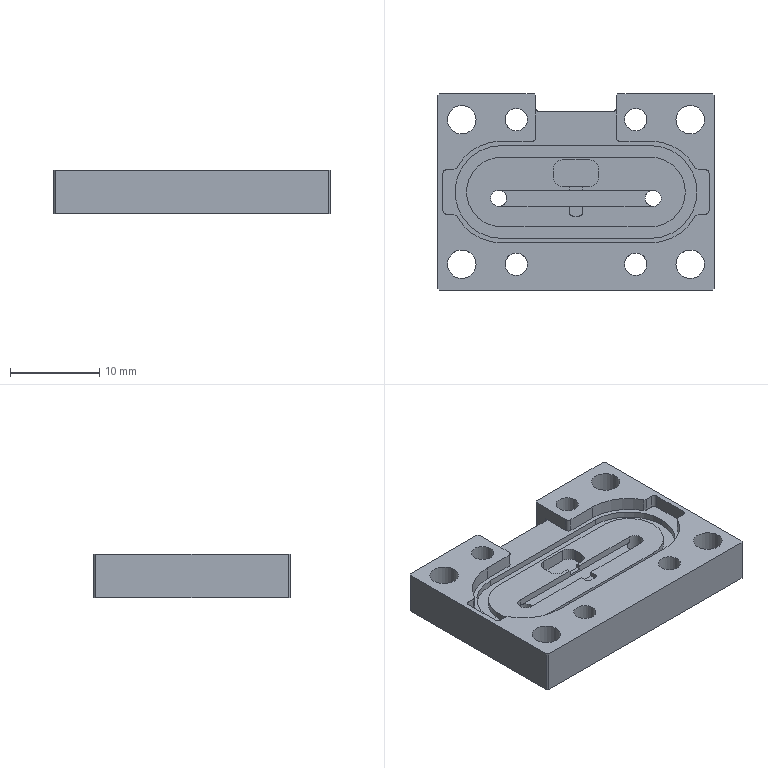NC program | NX | posted with a generic post | part box 31 x 22 x 4.9 mm
Lines 1 to 1660 of 7945, first 1453 of 1628 lines:
N10 G17 G21 G94 G90
(FACE_MILLING , TOOL : D50面刀)
N12 T12 M6
N14 G54
N16 G17 G0 G90 X43.5 Y0. S1600 M3
N18 G43 Z20. H12
N20 Z2.525
N22 G94 G1 Z0.525 F600.
N24 X40.5
N26 X-40.5
N28 X-43.5
N30 Z2.525
N32 G0 Z20.
N34 X43.5
N36 Z2.05
N38 G1 Z0.05
N40 X40.5
N42 X-40.5
N44 X-43.5
N46 Z2.05
N48 G0 Z20.
N50 M5
(ADAPTIVE_MILLING , TOOL : 6C-15L-25L)
N52 T02 M6
N54 G54
N56 G17 G0 G90 X-22.07 Y-0.418 S4500 M3
N58 G43 Z20. H2
N60 Z-2.9
N62 G94 G1 Z-5.9 F1500.
N64 X-21.095 Y-0.409
N66 G3 X-20.53 Y-0.006 R0.608
N68 X-20.23 Y2.844 R10.658
N70 G2 X-20.172 Y12.116 R798.279
N72 X-17.608 Y15.015 R3.885
N74 X-13.478 Y15.659 R12.183
N76 G1 X-7.365 Y15.7
N78 X16.28 Y15.698
N80 G2 X19.379 Y13.415 R3.673
N82 X20.139 Y9.502 R10.224
N84 X20.172 Y-12.09 R928.263
N86 X17.539 Y-15.024 R3.915
N88 X13.407 Y-15.647 R12.574
N90 G1 X7.369 Y-15.688
N92 X-16.328 Y-15.696
N94 G2 X-19.386 Y-13.414 R3.675
N96 X-20.146 Y-9.35 R10.554
N98 X-20.141 Y-0.409 R126.129
N100 G3 X-19.9 Y7.956 R92.469
N102 G2 X-19.829 Y11.214 R25.556
N104 X-16.647 Y14.675 R4.74
N106 X-11.881 Y15.361 R14.905
N108 G1 X-5.656 Y15.399
N110 X15.004 Y15.398
N112 G2 X19.076 Y12.392 R4.554
N114 X19.847 Y7.794 R13.145
N116 X19.876 Y-10.853 R799.951
N118 X16.799 Y-14.599 R4.632
N120 X12.304 Y-15.333 R13.408
N122 X5.592 Y-15.388 R559.777
N124 G1 X-15.015 Y-15.397
N126 G2 X-19.054 Y-12.451 R4.529
N128 X-19.846 Y-7.818 R12.948
N130 X-19.675 Y2.314 R100.736
N132 G1 X-19.576 Y9.907
N134 G2 X-16.059 Y14.284 R5.172
N136 X-11.378 Y15.039 R14.663
N138 X-3.804 Y15.099 R572.181
N140 G1 X13.955 Y15.097
N142 G2 X18.731 Y11.687 R5.128
N144 X19.534 Y6.98 R14.045
N146 X19.565 Y-9.99 R503.525
N148 X16.034 Y-14.277 R5.19
N150 X11.051 Y-15.036 R15.491
N152 G1 X3.777 Y-15.089
N154 X-13.961 Y-15.095
N156 G2 X-18.749 Y-11.651 R5.129
N158 X-19.543 Y-6.75 R14.635
N160 X-19.376 Y2.491 R107.625
N162 X-19.256 Y9.274 R367.832
N164 X-18.556 Y11.514 R6.868
N166 X-15.459 Y14.198 R3.677
N168 X-8.897 Y14.778 R31.595
N170 G1 X-2.597 Y14.799
N172 G2 X13.64 Y14.771 R937.515
N174 X16.022 Y14.055 R7.126
N176 X18.648 Y11.178 R3.618
N178 X19.278 Y4.359 R31.12
N180 X19.266 Y-9.177 R445.151
N182 X18.559 Y-11.492 R6.838
N184 X15.604 Y-14.161 R3.602
N186 X8.519 Y-14.77 R33.556
N188 G1 X3.419 Y-14.789
N190 X-12.915 Y-14.795
N192 G2 X-16.018 Y-14.056 R6.813
N194 X-18.698 Y-10.959 R3.68
N196 X-19.28 Y-4.022 R32.852
N198 X-19.034 Y4.585 R641.476
N200 X-18.917 Y8.867 R47.436
N202 G1 X-18.65 Y10.111
N204 G2 X-18.228 Y12.375 R3.99
N206 X-16.115 Y14.043 R3.859
N208 X-6.563 Y14.49 R80.605
N210 G1 X-1.538 Y14.499
N212 G2 X13.385 Y14.472 R874.725
N214 G1 X14.709 Y14.15
N216 G2 X16.045 Y14.052 R7.674
N218 G3 X16.699 Y14.816 R0.6
N220 X16.308 Y15.245 Z-5.85 R0.784
N222 G1 X15.815 Y15.573 Z-5.8
N224 X15.129 Y16.022
N226 X15.004 Y16.06
N228 X14.874 Y16.08
N230 X-14.033 Y16.171
N232 X-14.165 Y16.13
N234 X-14.289 Y16.068
N236 X-14.879 Y15.649
N238 X-15.23 Y15.408 Z-5.836
N240 X-15.563 Y15.142 Z-5.872
N242 X-15.653 Y15.001 Z-5.886
N244 X-15.704 Y14.842 Z-5.9
N246 G3 X-15.111 Y14.15 R0.6
N248 G1 X-3.186 Y14.197
N250 X12.714 Y14.198
N252 G3 X14.735 Y14.15 R11.377
N254 X14.943 Y15.313 R0.6
N256 G1 X13.797 Y15.63 Z-5.8
N258 X13.442 Y15.734
N260 X13.079 Y15.806
N262 X-7.985 Y15.8
N264 X-8.577 Y15.643
N266 X-9.723 Y15.327 Z-5.9
N268 G3 X-9.561 Y14.15 R0.6
N270 G1 X-4.698
N272 G3 X0.873 Y13.901 R37.444
N274 X3.621 Y13.934 R28.005
N276 G2 X4.702 Y14.15 R3.288
N278 G1 X13.064
N280 G3 X13.724 Y14.81 R0.66
N282 X13.058 Y15.47 R0.66
N284 G1 X4.434 Y15.389
N286 X3.245 Y15.377 Z-5.8
N288 X-3.054 Y15.318
N290 X-3.421 Z-5.831
N292 X-3.788 Y15.292 Z-5.862
N294 G3 X-4.16 Y15.049 Z-5.9 R0.678
N296 X-3.885 Y14.043 R0.66
N298 X-0.878 Y13.646 R9.579
N300 X2.956 Y13.646 R38.958
N302 G1 X3.093 Y13.706
N304 G3 X3.325 Y14.534 R0.661
N306 X2.657 Y14.92 Z-5.831 R0.697
N308 G1 X2.287 Y14.94 Z-5.8
N310 X-2.826 Y15.22
N312 X-3.211 Y15.244 Z-5.832
N314 X-3.596 Y15.245 Z-5.865
N316 G3 X-3.962 Y15.06 Z-5.9 R0.687
N318 X-3.746 Y13.985 R0.66
N320 X-0.769 Y13.391 R7.752
N322 X2.624 Y13.404 R16.695
N324 X3.125 Y13.728 R3.317
N326 G1 X3.645 Y13.943
N328 G3 X3.915 Y14.956 R0.66
N330 X3.262 Y15.21 Z-5.838 R0.713
N332 G1 X2.806 Y15.199 Z-5.8
N334 X-2.47 Y15.068
N336 X-2.826 Y15.063 Z-5.83
N338 X-3.181 Y15.029 Z-5.86
N340 G3 X-3.559 Y14.758 Z-5.9 R0.674
N342 X-3.261 Y13.784 R0.66
N344 X-0.251 Y13.116 R7.191
N346 X2.371 Y13.18 R8.911
N348 G1 X2.826 Y13.499
N350 G3 X3.017 Y14.314 R0.661
N352 X2.347 Y14.686 Z-5.832 R0.698
N354 G1 X1.971 Y14.703 Z-5.8
N356 X-2.179 Y14.888
N358 X-2.508 Y14.905 Z-5.828
N360 X-2.837 Y14.9 Z-5.856
N362 G3 X-3.27 Y14.62 Z-5.9 R0.669
N364 X-3.125 Y13.728 R0.661
N366 X-0.846 Y12.948 R4.437
N368 X2.118 Y12.95 R7.962
N370 X2.501 Y13.249 R3.333
N372 X2.698 Y14.052 R0.661
N374 X2.037 Y14.439 Z-5.832 R0.699
N376 G1 X1.66 Y14.465 Z-5.8
N378 X-1.954 Y14.714
N380 X-2.283 Y14.74 Z-5.828
N382 X-2.613 Y14.743 Z-5.856
N384 G3 X-3.052 Y14.475 Z-5.9 R0.669
N386 X-2.917 Y13.568 R0.661
N388 X-0.467 Y12.683 R4.638
N390 X2.018 Y12.784 R5.044
N392 G1 X2.334 Y13.085
N394 G3 X2.452 Y13.837 R0.662
N396 X1.802 Y14.212 Z-5.833 R0.704
N398 G1 X1.407 Y14.245 Z-5.8
N400 X-1.68 Y14.501
N402 X-2.007 Y14.531 Z-5.828
N404 X-2.337 Y14.538 Z-5.856
N406 G3 X-2.78 Y14.276 Z-5.9 R0.668
N408 X-2.649 Y13.363 R0.661
N410 X0.082 Y12.41 R4.757
N412 X1.904 Y12.62 R3.297
N414 G1 X2.175 Y12.911
N416 G3 X2.275 Y13.642 R0.662
N418 X1.629 Y14.019 Z-5.834 R0.705
N420 G1 X1.231 Y14.055 Z-5.8
N422 X-1.435 Y14.298
N424 X-1.759 Y14.33 Z-5.827
N426 X-2.085 Y14.339 Z-5.855
N428 G3 X-2.533 Y14.074 Z-5.9 R0.668
N430 X-2.472 Y13.226 R0.661
N432 X-0.241 Y12.252 R3.679
N434 X1.777 Y12.447 R3.122
N436 G1 X1.906 Y12.582
N438 G3 X1.934 Y13.214 R0.665
N440 X1.35 Y13.593 Z-5.839 R0.715
N442 G1 X0.896 Y13.679 Z-5.8
N444 X-1.217 Y14.079
N446 X-1.538 Y14.142 Z-5.828
N448 X-1.864 Y14.183 Z-5.855
N450 G3 X-2.333 Y13.966 Z-5.9 R0.668
N452 X-2.315 Y13.065 R0.661
N454 X-0.59 Y12.15 R2.983
N456 X1.471 Y12.211 R10.87
N458 X1.998 Y12.704 R1.047
N460 X2.074 Y13.424 R0.663
N462 X1.418 Y13.788 Z-5.833 R0.704
N464 G1 X1.022 Y13.814 Z-5.8
N466 X-1.099 Y13.955
N468 X-1.431 Y13.979 Z-5.828
N470 X-1.763 Y13.982 Z-5.856
N472 G3 X-2.199 Y13.718 Z-5.9 R0.669
N474 X-2.156 Y12.891 R0.661
N476 X-0.568 Y12.15 R1.703
N478 X-0.353 Y13.434 R0.66
N480 G1 X-1.382 Y13.78
N482 G3 X-2.004 Y12.712 R0.66
N484 X-1. Y12.15 R1.075
N486 X-0.759 Y13.425 R0.66
N488 G1 X-1.221 Y13.595
N490 G3 X-1.927 Y12.617 R0.66
N492 X-1.224 Y12.15 R0.744
N494 X-1.896 Y13.122 R-0.713
N496 X-1.851 Y12.487 R0.727
N498 X-1.299 Y12.15 R0.666
N500 G1 X1.427 Y12.163
N502 G3 X1.852 Y12.489 R0.739
N504 X1.912 Y12.953 R0.615
N506 G1 X1.839 Y13.214
N508 X1.521 Y14.359 Z-5.8
N510 G2 X1.852 Y15.165 R0.613
N512 G1 X2.711 Y15.512
N514 X3.584 Y15.822
N516 X3.944 Y15.906
N518 X4.31 Y15.951
N520 X7.639 Y16.145
N522 X10.969 Y16.318
N524 G2 X15.315 Y16.024 R22.708
N526 G1 X16.999 Y15.737
N528 G2 X18.51 Y14.907 R3.241
N530 G1 X19.297 Y14.13
N532 G2 X19.318 Y13.431 R0.619
N534 G1 X18.796 Y12.362 Z-5.9
N536 X18.655 Y12.083
N538 G3 X18.543 Y11.615 R1.223
N540 G2 X18.99 Y1.939 R81.107
N542 X18.972 Y-8.859 R673.915
N544 G1 X18.65 Y-10.196
N546 G2 X18.557 Y-11.508 R7.62
N548 G3 X19.321 Y-12.162 R0.6
N550 X19.75 Y-11.771 Z-5.85 R0.784
N552 G1 X20.078 Y-11.277 Z-5.8
N554 X20.527 Y-10.591
N556 X20.565 Y-10.466
N558 X20.585 Y-10.337
N560 X20.671 Y9.495
N562 X20.63 Y9.628
N564 X20.567 Y9.752
N566 X20.149 Y10.342
N568 X19.908 Y10.693 Z-5.836
N570 X19.642 Y11.025 Z-5.872
N572 X19.501 Y11.115 Z-5.886
N574 X19.342 Y11.166 Z-5.9
N576 G3 X18.65 Y10.573 R0.6
N578 G1 X18.697 Y-1.545
N580 G2 X18.65 Y-10.203 R441.565
N582 G3 X19.813 Y-10.412 R0.6
N584 G1 X20.13 Y-9.266 Z-5.8
N586 X20.234 Y-8.911
N588 X20.306 Y-8.548
N590 X20.3 Y3.373
N592 X20.143 Y3.964
N594 X19.828 Y5.111 Z-5.9
N596 G3 X18.65 Y4.948 R0.6
N598 G1 Y-10.802
N600 G2 X14.91 Y-14.153 R3.498
N602 X3.692 Y-14.481 R128.863
N604 G1 X-0.808 Y-14.491
N606 G2 X-13.363 Y-14.47 R602.67
N608 G1 X-14.703 Y-14.15
N610 G2 X-16.045 Y-14.052 R7.665
N612 G3 X-16.699 Y-14.816 R0.6
N614 X-16.308 Y-15.245 Z-5.85 R0.784
N616 G1 X-15.815 Y-15.573 Z-5.8
N618 X-15.129 Y-16.022
N620 X-15.004 Y-16.06
N622 X-14.874 Y-16.08
N624 X13.92 Y-16.171
N626 X14.053 Y-16.13
N628 X14.176 Y-16.068
N630 X14.767 Y-15.649
N632 X15.118 Y-15.408 Z-5.836
N634 X15.45 Y-15.142 Z-5.872
N636 X15.54 Y-15.001 Z-5.886
N638 X15.591 Y-14.842 Z-5.9
N640 G3 X14.998 Y-14.15 R0.6
N642 G1 X-0.945 Y-14.19
N644 G2 X-14.706 Y-14.15 R831.508
N646 G3 X-14.915 Y-15.313 R0.6
N648 G1 X-13.769 Y-15.63 Z-5.8
N650 X-13.413 Y-15.734
N652 X-13.051 Y-15.806
N654 X4.273 Y-15.8
N656 X4.864 Y-15.643
N658 X6.011 Y-15.328 Z-5.9
N660 G3 X5.848 Y-14.15 R0.6
N662 G1 X-15.302
N664 G2 X-18.657 Y-10.406 R3.505
N666 X-18.81 Y1.708 R84.207
N668 G3 X-18.65 Y10.14 R365.879
N670 X-19.815 Y10.341 R0.6
N672 G1 X-20.13 Y9.194 Z-5.8
N674 X-20.231 Y8.842
N676 X-20.306 Y8.484
N678 X-20.678 Y-9.442
N680 X-20.65 Y-9.631
N682 X-20.566 Y-9.803
N684 X-20.152 Y-10.383
N686 X-19.908 Y-10.733 Z-5.836
N688 X-19.64 Y-11.066 Z-5.872
N690 X-19.5 Y-11.155 Z-5.886
N692 X-19.342 Y-11.205 Z-5.9
N694 G3 X-18.65 Y-10.613 R0.6
N696 G1 Y7.988
N698 G3 X-19.36 Y8.584 R0.606
N700 G1 X-20.137 Y8.449
N702 Z-2.9
N704 G0 Z20.
N706 M5
(DRILLING , TOOL : D5点钻)
N708 T07 M6
N710 G54
N712 G17 G0 G90 X-12.8 Y8.1 S1200 M3
N714 G43 Z20. H7
N716 G94 G81 G99 Z-1. F100. R3.
N718 X-6.7
N720 X6.7
N722 X12.8
N724 Y-8.1
N726 X6.7
N728 X-6.7
N730 X-12.8
N732 G80
N734 G0 X-12.8 Y-8.1 Z20.
N736 M5
(DRILLING_1 , TOOL : D3.2钻头)
N738 T08 M6
N740 G54
N742 G17 G0 G90 X-12.8 Y8.1 S1600 M3
N744 G43 Z20. H8
N746 G94 G83 G99 Z-7.361 F80. Q1. R3.
N748 Y-8.1
N750 X12.8
N752 Y8.1
N754 G80
N756 G0 X12.8 Y8.1 Z20.
N758 M5
(DRILLING_2 , TOOL : D2.5钻头)
N760 T13 M6
N762 G54
N764 G17 G0 G90 X-6.7 Y8.1 S3000 M3
N766 G43 Z20. H13
N768 G94 G81 G99 Z-6.5 F60. R3.
N770 X6.7
N772 Y-8.1
N774 X-6.7
N776 G80
N778 G0 X-6.7 Y-8.1 Z20.
N780 M5
(DRILLING_COPY , TOOL : D5点钻)
N782 T07 M6
N784 G54
N786 G17 G0 G90 X-12.8 Y8.1 S2000 M3
N788 G43 Z20. H7
N790 G94 G81 G99 Z-1.6 F80. R3.
N792 X12.8
N794 Y-8.1
N796 X-12.8
N798 G80
N800 G0 X-12.8 Y-8.1 Z20.
(DRILLING_COPY_1 , TOOL : D5点钻)
N802 X-6.7 Y8.1
N804 G81 Z-1.4 F80. R3.
N806 X6.7
N808 Y-8.1
N810 X-6.7
N812 G80
N814 G0 X-6.7 Y-8.1 Z20.
N816 M5
(THREAD_MILLING , TOOL : 螺纹铣刀M3)
N818 T14 M6
N820 G54
N822 G17 G0 G90 X-6.7 Y8.1 S3500 M3
N824 G43 Z20. H14
N826 Z0.625
N828 G42 G94 G1 X-6.713 Y8.035 Z0.583 F80. D14
N830 X-6.788 Z0.542
N832 X-6.8 Y8.1 Z0.5
N834 G2 X-6.8 Y8.1 Z0. I0.1 J0.
N836 X-6.8 Y8.1 Z-0.5 I0.1 J0.
N838 X-6.8 Y8.1 Z-1. I0.1 J0.
N840 X-6.8 Y8.1 Z-1.5 I0.1 J0.
N842 X-6.8 Y8.1 Z-2. I0.1 J0.
N844 X-6.8 Y8.1 Z-2.5 I0.1 J0.
N846 X-6.8 Y8.1 Z-3. I0.1 J0.
N848 X-6.8 Y8.1 Z-3.5 I0.1 J0.
N850 X-6.8 Y8.1 Z-4. I0.1 J0.
N852 X-6.8 Y8.1 Z-4.5 I0.1 J0.
N854 X-6.8 Y8.1 Z-5. I0.1 J0.
N856 X-6.8 Y8.1 Z-5.5 I0.1 J0.
N858 X-6.731 Y8.195 Z-5.6 R0.1
N860 G1 X-6.665 Y8.203 Z-5.642
N862 X-6.642 Y8.132 Z-5.683
N864 X-6.7 Y8.1 Z-5.725
N866 G40
N868 G0 Z20.
N870 Z0.547
N872 G42 G1 X-6.789 Y8.055
N874 X-6.826 Y8.033 Z0.531
N876 X-6.86 Y8.059 Z0.516
N878 X-6.85 Y8.1 Z0.5
N880 G2 X-6.85 Y8.1 Z0. I0.15 J0.
N882 X-6.85 Y8.1 Z-0.5 I0.15 J0.
N884 X-6.85 Y8.1 Z-1. I0.15 J0.
N886 X-6.85 Y8.1 Z-1.5 I0.15 J0.
N888 X-6.85 Y8.1 Z-2. I0.15 J0.
N890 X-6.85 Y8.1 Z-2.5 I0.15 J0.
N892 X-6.85 Y8.1 Z-3. I0.15 J0.
N894 X-6.85 Y8.1 Z-3.5 I0.15 J0.
N896 X-6.85 Y8.1 Z-4. I0.15 J0.
N898 X-6.85 Y8.1 Z-4.5 I0.15 J0.
N900 X-6.85 Y8.1 Z-5. I0.15 J0.
N902 X-6.85 Y8.1 Z-5.5 I0.15 J0.
N904 X-6.746 Y8.243 Z-5.6 R0.15
N906 G1 X-6.71 Y8.265 Z-5.616
N908 X-6.675 Y8.24 Z-5.631
N910 X-6.685 Y8.199 Z-5.647
N912 G40
N914 X-6.7 Y8.1
N916 G0 Z20.
N918 Z0.57
N920 G42 G1 X-6.773 Y8.031
N922 X-6.833 Y7.989 Z0.547
N924 X-6.902 Y8.026 Z0.523
N926 X-6.9 Y8.1 Z0.5
N928 G2 X-6.9 Y8.1 Z0. I0.2 J0.
N930 X-6.9 Y8.1 Z-0.5 I0.2 J0.
N932 X-6.9 Y8.1 Z-1. I0.2 J0.
N934 X-6.9 Y8.1 Z-1.5 I0.2 J0.
N936 X-6.9 Y8.1 Z-2. I0.2 J0.
N938 X-6.9 Y8.1 Z-2.5 I0.2 J0.
N940 X-6.9 Y8.1 Z-3. I0.2 J0.
N942 X-6.9 Y8.1 Z-3.5 I0.2 J0.
N944 X-6.9 Y8.1 Z-4. I0.2 J0.
N946 X-6.9 Y8.1 Z-4.5 I0.2 J0.
N948 X-6.9 Y8.1 Z-5. I0.2 J0.
N950 X-6.9 Y8.1 Z-5.5 I0.2 J0.
N952 X-6.762 Y8.29 Z-5.6 R0.2
N954 G1 X-6.692 Y8.315 Z-5.623
N956 X-6.635 Y8.261 Z-5.647
N958 X-6.657 Y8.19 Z-5.67
N960 G40
N962 X-6.7 Y8.1
N964 G0 Z20.
N966 Z0.584
N968 G42 G1 X-6.759 Y8.019
N970 G2 X-6.95 Y8.1 Z0.5 R0.113
N972 X-6.95 Y8.1 Z0. I0.25 J0.
N974 X-6.95 Y8.1 Z-0.5 I0.25 J0.
N976 X-6.95 Y8.1 Z-1. I0.25 J0.
N978 X-6.95 Y8.1 Z-1.5 I0.25 J0.
N980 X-6.95 Y8.1 Z-2. I0.25 J0.
N982 X-6.95 Y8.1 Z-2.5 I0.25 J0.
N984 X-6.95 Y8.1 Z-3. I0.25 J0.
N986 X-6.95 Y8.1 Z-3.5 I0.25 J0.
N988 X-6.95 Y8.1 Z-4. I0.25 J0.
N990 X-6.95 Y8.1 Z-4.5 I0.25 J0.
N992 X-6.95 Y8.1 Z-5. I0.25 J0.
N994 X-6.95 Y8.1 Z-5.5 I0.25 J0.
N996 X-6.777 Y8.338 Z-5.6 R0.25
N998 X-6.641 Y8.181 Z-5.684 R0.113
N1000 G40
N1002 G1 X-6.7 Y8.1
N1004 G0 Z20.
N1006 X6.7
N1008 Z0.625
N1010 G42 G1 X6.713 Y8.165 Z0.583
N1012 X6.788 Z0.542
N1014 X6.8 Y8.1 Z0.5
N1016 G2 X6.8 Y8.1 Z0. I-0.1 J0.
N1018 X6.8 Y8.1 Z-0.5 I-0.1 J0.
N1020 X6.8 Y8.1 Z-1. I-0.1 J0.
N1022 X6.8 Y8.1 Z-1.5 I-0.1 J0.
N1024 X6.8 Y8.1 Z-2. I-0.1 J0.
N1026 X6.8 Y8.1 Z-2.5 I-0.1 J0.
N1028 X6.8 Y8.1 Z-3. I-0.1 J0.
N1030 X6.8 Y8.1 Z-3.5 I-0.1 J0.
N1032 X6.8 Y8.1 Z-4. I-0.1 J0.
N1034 X6.8 Y8.1 Z-4.5 I-0.1 J0.
N1036 X6.8 Y8.1 Z-5. I-0.1 J0.
N1038 X6.8 Y8.1 Z-5.5 I-0.1 J0.
N1040 X6.731 Y8.005 Z-5.6 R0.1
N1042 G1 X6.665 Y7.997 Z-5.642
N1044 X6.642 Y8.068 Z-5.683
N1046 X6.7 Y8.1 Z-5.725
N1048 G40
N1050 G0 Z20.
N1052 Z0.547
N1054 G42 G1 X6.789 Y8.145
N1056 X6.826 Y8.167 Z0.531
N1058 X6.86 Y8.141 Z0.516
N1060 X6.85 Y8.1 Z0.5
N1062 G2 X6.85 Y8.1 Z0. I-0.15 J0.
N1064 X6.85 Y8.1 Z-0.5 I-0.15 J0.
N1066 X6.85 Y8.1 Z-1. I-0.15 J0.
N1068 X6.85 Y8.1 Z-1.5 I-0.15 J0.
N1070 X6.85 Y8.1 Z-2. I-0.15 J0.
N1072 X6.85 Y8.1 Z-2.5 I-0.15 J0.
N1074 X6.85 Y8.1 Z-3. I-0.15 J0.
N1076 X6.85 Y8.1 Z-3.5 I-0.15 J0.
N1078 X6.85 Y8.1 Z-4. I-0.15 J0.
N1080 X6.85 Y8.1 Z-4.5 I-0.15 J0.
N1082 X6.85 Y8.1 Z-5. I-0.15 J0.
N1084 X6.85 Y8.1 Z-5.5 I-0.15 J0.
N1086 X6.746 Y7.957 Z-5.6 R0.15
N1088 G1 X6.71 Y7.935 Z-5.616
N1090 X6.675 Y7.96 Z-5.631
N1092 X6.685 Y8.001 Z-5.647
N1094 G40
N1096 X6.7 Y8.1
N1098 G0 Z20.
N1100 Z0.57
N1102 G42 G1 X6.773 Y8.169
N1104 X6.833 Y8.211 Z0.547
N1106 X6.902 Y8.174 Z0.523
N1108 X6.9 Y8.1 Z0.5
N1110 G2 X6.9 Y8.1 Z0. I-0.2 J0.
N1112 X6.9 Y8.1 Z-0.5 I-0.2 J0.
N1114 X6.9 Y8.1 Z-1. I-0.2 J0.
N1116 X6.9 Y8.1 Z-1.5 I-0.2 J0.
N1118 X6.9 Y8.1 Z-2. I-0.2 J0.
N1120 X6.9 Y8.1 Z-2.5 I-0.2 J0.
N1122 X6.9 Y8.1 Z-3. I-0.2 J0.
N1124 X6.9 Y8.1 Z-3.5 I-0.2 J0.
N1126 X6.9 Y8.1 Z-4. I-0.2 J0.
N1128 X6.9 Y8.1 Z-4.5 I-0.2 J0.
N1130 X6.9 Y8.1 Z-5. I-0.2 J0.
N1132 X6.9 Y8.1 Z-5.5 I-0.2 J0.
N1134 X6.762 Y7.91 Z-5.6 R0.2
N1136 G1 X6.692 Y7.885 Z-5.623
N1138 X6.635 Y7.939 Z-5.647
N1140 X6.657 Y8.01 Z-5.67
N1142 G40
N1144 X6.7 Y8.1
N1146 G0 Z20.
N1148 Z0.584
N1150 G42 G1 X6.759 Y8.181
N1152 G2 X6.95 Y8.1 Z0.5 R0.113
N1154 X6.95 Y8.1 Z0. I-0.25 J0.
N1156 X6.95 Y8.1 Z-0.5 I-0.25 J0.
N1158 X6.95 Y8.1 Z-1. I-0.25 J0.
N1160 X6.95 Y8.1 Z-1.5 I-0.25 J0.
N1162 X6.95 Y8.1 Z-2. I-0.25 J0.
N1164 X6.95 Y8.1 Z-2.5 I-0.25 J0.
N1166 X6.95 Y8.1 Z-3. I-0.25 J0.
N1168 X6.95 Y8.1 Z-3.5 I-0.25 J0.
N1170 X6.95 Y8.1 Z-4. I-0.25 J0.
N1172 X6.95 Y8.1 Z-4.5 I-0.25 J0.
N1174 X6.95 Y8.1 Z-5. I-0.25 J0.
N1176 X6.95 Y8.1 Z-5.5 I-0.25 J0.
N1178 X6.777 Y7.862 Z-5.6 R0.25
N1180 X6.641 Y8.019 Z-5.684 R0.113
N1182 G40
N1184 G1 X6.7 Y8.1
N1186 G0 Z20.
N1188 Y-8.1
N1190 Z0.625
N1192 G42 G1 X6.713 Y-8.035 Z0.583
N1194 X6.788 Z0.542
N1196 X6.8 Y-8.1 Z0.5
N1198 G2 X6.8 Y-8.1 Z0. I-0.1 J0.
N1200 X6.8 Y-8.1 Z-0.5 I-0.1 J0.
N1202 X6.8 Y-8.1 Z-1. I-0.1 J0.
N1204 X6.8 Y-8.1 Z-1.5 I-0.1 J0.
N1206 X6.8 Y-8.1 Z-2. I-0.1 J0.
N1208 X6.8 Y-8.1 Z-2.5 I-0.1 J0.
N1210 X6.8 Y-8.1 Z-3. I-0.1 J0.
N1212 X6.8 Y-8.1 Z-3.5 I-0.1 J0.
N1214 X6.8 Y-8.1 Z-4. I-0.1 J0.
N1216 X6.8 Y-8.1 Z-4.5 I-0.1 J0.
N1218 X6.8 Y-8.1 Z-5. I-0.1 J0.
N1220 X6.8 Y-8.1 Z-5.5 I-0.1 J0.
N1222 X6.731 Y-8.195 Z-5.6 R0.1
N1224 G1 X6.665 Y-8.203 Z-5.642
N1226 X6.642 Y-8.132 Z-5.683
N1228 X6.7 Y-8.1 Z-5.725
N1230 G40
N1232 G0 Z20.
N1234 Z0.547
N1236 G42 G1 X6.789 Y-8.055
N1238 X6.826 Y-8.033 Z0.531
N1240 X6.86 Y-8.059 Z0.516
N1242 X6.85 Y-8.1 Z0.5
N1244 G2 X6.85 Y-8.1 Z0. I-0.15 J0.
N1246 X6.85 Y-8.1 Z-0.5 I-0.15 J0.
N1248 X6.85 Y-8.1 Z-1. I-0.15 J0.
N1250 X6.85 Y-8.1 Z-1.5 I-0.15 J0.
N1252 X6.85 Y-8.1 Z-2. I-0.15 J0.
N1254 X6.85 Y-8.1 Z-2.5 I-0.15 J0.
N1256 X6.85 Y-8.1 Z-3. I-0.15 J0.
N1258 X6.85 Y-8.1 Z-3.5 I-0.15 J0.
N1260 X6.85 Y-8.1 Z-4. I-0.15 J0.
N1262 X6.85 Y-8.1 Z-4.5 I-0.15 J0.
N1264 X6.85 Y-8.1 Z-5. I-0.15 J0.
N1266 X6.85 Y-8.1 Z-5.5 I-0.15 J0.
N1268 X6.746 Y-8.243 Z-5.6 R0.15
N1270 G1 X6.71 Y-8.265 Z-5.616
N1272 X6.675 Y-8.24 Z-5.631
N1274 X6.685 Y-8.199 Z-5.647
N1276 G40
N1278 X6.7 Y-8.1
N1280 G0 Z20.
N1282 Z0.57
N1284 G42 G1 X6.773 Y-8.031
N1286 X6.833 Y-7.989 Z0.547
N1288 X6.902 Y-8.026 Z0.523
N1290 X6.9 Y-8.1 Z0.5
N1292 G2 X6.9 Y-8.1 Z0. I-0.2 J0.
N1294 X6.9 Y-8.1 Z-0.5 I-0.2 J0.
N1296 X6.9 Y-8.1 Z-1. I-0.2 J0.
N1298 X6.9 Y-8.1 Z-1.5 I-0.2 J0.
N1300 X6.9 Y-8.1 Z-2. I-0.2 J0.
N1302 X6.9 Y-8.1 Z-2.5 I-0.2 J0.
N1304 X6.9 Y-8.1 Z-3. I-0.2 J0.
N1306 X6.9 Y-8.1 Z-3.5 I-0.2 J0.
N1308 X6.9 Y-8.1 Z-4. I-0.2 J0.
N1310 X6.9 Y-8.1 Z-4.5 I-0.2 J0.
N1312 X6.9 Y-8.1 Z-5. I-0.2 J0.
N1314 X6.9 Y-8.1 Z-5.5 I-0.2 J0.
N1316 X6.762 Y-8.29 Z-5.6 R0.2
N1318 G1 X6.692 Y-8.315 Z-5.623
N1320 X6.635 Y-8.261 Z-5.647
N1322 X6.657 Y-8.19 Z-5.67
N1324 G40
N1326 X6.7 Y-8.1
N1328 G0 Z20.
N1330 Z0.584
N1332 G42 G1 X6.759 Y-8.019
N1334 G2 X6.95 Y-8.1 Z0.5 R0.113
N1336 X6.95 Y-8.1 Z0. I-0.25 J0.
N1338 X6.95 Y-8.1 Z-0.5 I-0.25 J0.
N1340 X6.95 Y-8.1 Z-1. I-0.25 J0.
N1342 X6.95 Y-8.1 Z-1.5 I-0.25 J0.
N1344 X6.95 Y-8.1 Z-2. I-0.25 J0.
N1346 X6.95 Y-8.1 Z-2.5 I-0.25 J0.
N1348 X6.95 Y-8.1 Z-3. I-0.25 J0.
N1350 X6.95 Y-8.1 Z-3.5 I-0.25 J0.
N1352 X6.95 Y-8.1 Z-4. I-0.25 J0.
N1354 X6.95 Y-8.1 Z-4.5 I-0.25 J0.
N1356 X6.95 Y-8.1 Z-5. I-0.25 J0.
N1358 X6.95 Y-8.1 Z-5.5 I-0.25 J0.
N1360 X6.777 Y-8.338 Z-5.6 R0.25
N1362 X6.641 Y-8.181 Z-5.684 R0.113
N1364 G40
N1366 G1 X6.7 Y-8.1
N1368 G0 Z20.
N1370 X-6.7
N1372 Z0.625
N1374 G42 G1 X-6.688 Y-8.035 Z0.583
N1376 X-6.613 Z0.542
N1378 X-6.6 Y-8.1 Z0.5
N1380 G2 X-6.6 Y-8.1 Z0. I-0.1 J0.
N1382 X-6.6 Y-8.1 Z-0.5 I-0.1 J0.
N1384 X-6.6 Y-8.1 Z-1. I-0.1 J0.
N1386 X-6.6 Y-8.1 Z-1.5 I-0.1 J0.
N1388 X-6.6 Y-8.1 Z-2. I-0.1 J0.
N1390 X-6.6 Y-8.1 Z-2.5 I-0.1 J0.
N1392 X-6.6 Y-8.1 Z-3. I-0.1 J0.
N1394 X-6.6 Y-8.1 Z-3.5 I-0.1 J0.
N1396 X-6.6 Y-8.1 Z-4. I-0.1 J0.
N1398 X-6.6 Y-8.1 Z-4.5 I-0.1 J0.
N1400 X-6.6 Y-8.1 Z-5. I-0.1 J0.
N1402 X-6.6 Y-8.1 Z-5.5 I-0.1 J0.
N1404 X-6.669 Y-8.195 Z-5.6 R0.1
N1406 G1 X-6.735 Y-8.203 Z-5.642
N1408 X-6.758 Y-8.132 Z-5.683
N1410 X-6.7 Y-8.1 Z-5.725
N1412 G40
N1414 G0 Z20.
N1416 Z0.547
N1418 G42 G1 X-6.611 Y-8.055
N1420 X-6.574 Y-8.033 Z0.531
N1422 X-6.54 Y-8.059 Z0.516
N1424 X-6.55 Y-8.1 Z0.5
N1426 G2 X-6.55 Y-8.1 Z0. I-0.15 J0.
N1428 X-6.55 Y-8.1 Z-0.5 I-0.15 J0.
N1430 X-6.55 Y-8.1 Z-1. I-0.15 J0.
N1432 X-6.55 Y-8.1 Z-1.5 I-0.15 J0.
N1434 X-6.55 Y-8.1 Z-2. I-0.15 J0.
N1436 X-6.55 Y-8.1 Z-2.5 I-0.15 J0.
N1438 X-6.55 Y-8.1 Z-3. I-0.15 J0.
N1440 X-6.55 Y-8.1 Z-3.5 I-0.15 J0.
N1442 X-6.55 Y-8.1 Z-4. I-0.15 J0.
N1444 X-6.55 Y-8.1 Z-4.5 I-0.15 J0.
N1446 X-6.55 Y-8.1 Z-5. I-0.15 J0.
N1448 X-6.55 Y-8.1 Z-5.5 I-0.15 J0.
N1450 X-6.654 Y-8.243 Z-5.6 R0.15
N1452 G1 X-6.69 Y-8.265 Z-5.616
N1454 X-6.725 Y-8.24 Z-5.631
N1456 X-6.715 Y-8.199 Z-5.647
N1458 G40
N1460 X-6.7 Y-8.1
N1462 G0 Z20.
N1464 Z0.57
N1466 G42 G1 X-6.627 Y-8.031
N1468 X-6.567 Y-7.989 Z0.547
N1470 X-6.498 Y-8.026 Z0.523
N1472 X-6.5 Y-8.1 Z0.5
N1474 G2 X-6.5 Y-8.1 Z0. I-0.2 J0.
N1476 X-6.5 Y-8.1 Z-0.5 I-0.2 J0.
N1478 X-6.5 Y-8.1 Z-1. I-0.2 J0.
N1480 X-6.5 Y-8.1 Z-1.5 I-0.2 J0.
N1482 X-6.5 Y-8.1 Z-2. I-0.2 J0.
N1484 X-6.5 Y-8.1 Z-2.5 I-0.2 J0.
N1486 X-6.5 Y-8.1 Z-3. I-0.2 J0.
N1488 X-6.5 Y-8.1 Z-3.5 I-0.2 J0.
N1490 X-6.5 Y-8.1 Z-4. I-0.2 J0.
N1492 X-6.5 Y-8.1 Z-4.5 I-0.2 J0.
N1494 X-6.5 Y-8.1 Z-5. I-0.2 J0.
N1496 X-6.5 Y-8.1 Z-5.5 I-0.2 J0.
N1498 X-6.638 Y-8.29 Z-5.6 R0.2
N1500 G1 X-6.708 Y-8.315 Z-5.623
N1502 X-6.765 Y-8.261 Z-5.647
N1504 X-6.743 Y-8.19 Z-5.67
N1506 G40
N1508 X-6.7 Y-8.1
N1510 G0 Z20.
N1512 Z0.584
N1514 G42 G1 X-6.641 Y-8.019
N1516 G2 X-6.45 Y-8.1 Z0.5 R0.113
N1518 X-6.45 Y-8.1 Z0. I-0.25 J0.
N1520 X-6.45 Y-8.1 Z-0.5 I-0.25 J0.
N1522 X-6.45 Y-8.1 Z-1. I-0.25 J0.
N1524 X-6.45 Y-8.1 Z-1.5 I-0.25 J0.
N1526 X-6.45 Y-8.1 Z-2. I-0.25 J0.
N1528 X-6.45 Y-8.1 Z-2.5 I-0.25 J0.
N1530 X-6.45 Y-8.1 Z-3. I-0.25 J0.
N1532 X-6.45 Y-8.1 Z-3.5 I-0.25 J0.
N1534 X-6.45 Y-8.1 Z-4. I-0.25 J0.
N1536 X-6.45 Y-8.1 Z-4.5 I-0.25 J0.
N1538 X-6.45 Y-8.1 Z-5. I-0.25 J0.
N1540 X-6.45 Y-8.1 Z-5.5 I-0.25 J0.
N1542 X-6.623 Y-8.338 Z-5.6 R0.25
N1544 X-6.759 Y-8.181 Z-5.684 R0.113
N1546 G40
N1548 G1 X-6.7 Y-8.1
N1550 G0 Z20.
N1552 M5
(PLANAR_MILL , TOOL : 5J-15L-25L)
N1554 T03 M6
N1556 G54
N1558 G17 G0 G90 X2.2 Y16. S3000 M3
N1560 G43 Z20. H3
N1562 Z-2.9
N1564 G94 G1 Z-5.9 F400.
N1566 G41 Y13.5 D3
N1568 X4.7
N1570 X15.3
N1572 G2 X17.068 Y12.768 R2.5
N1574 G1 X17.268 Y12.568
N1576 G2 X18. Y10.8 R2.5
N1578 G1 Y-10.8
N1580 G2 X17.268 Y-12.568 R2.5
N1582 G1 X17.068 Y-12.768
N1584 G2 X15.3 Y-13.5 R2.5
N1586 G1 X-15.3
N1588 G2 X-17.068 Y-12.768 R2.5
N1590 G1 X-17.268 Y-12.568
N1592 G2 X-18. Y-10.8 R2.5
N1594 G1 Y10.8
N1596 G2 X-17.268 Y12.568 R2.5
N1598 G1 X-17.068 Y12.768
N1600 G2 X-15.3 Y13.5 R2.5
N1602 G1 X-4.7
N1604 X-2.2
N1606 G40
N1608 Y16.
N1610 Z-2.9
N1612 G0 Z20.
N1614 X2.2
N1616 Z-2.9
N1618 G1 Z-5.9
N1620 G41 Y13.5
N1622 X4.7
N1624 X15.3
N1626 G2 X17.068 Y12.768 R2.5
N1628 G1 X17.268 Y12.568
N1630 G2 X18. Y10.8 R2.5
N1632 G1 Y-10.8
N1634 G2 X17.268 Y-12.568 R2.5
N1636 G1 X17.068 Y-12.768
N1638 G2 X15.3 Y-13.5 R2.5
N1640 G1 X-15.3
N1642 G2 X-17.068 Y-12.768 R2.5
N1644 G1 X-17.268 Y-12.568
N1646 G2 X-18. Y-10.8 R2.5
N1648 G1 Y10.8
N1650 G2 X-17.268 Y12.568 R2.5
N1652 G1 X-17.068 Y12.768
N1654 G2 X-15.3 Y13.5 R2.5
N1656 G1 X-4.7
N1658 X-2.2
N1660 G40
N1662 Y16.
N1664 Z-2.9
N1666 G0 Z20.
N1668 X2.2
N1670 Z-2.9
N1672 G1 Z-5.9
N1674 G41 Y13.5
N1676 X4.7
N1678 X15.3
N1680 G2 X17.068 Y12.768 R2.5
N1682 G1 X17.268 Y12.568
N1684 G2 X18. Y10.8 R2.5
N1686 G1 Y-10.8
N1688 G2 X17.268 Y-12.568 R2.5
N1690 G1 X17.068 Y-12.768
N1692 G2 X15.3 Y-13.5 R2.5
N1694 G1 X-15.3
N1696 G2 X-17.068 Y-12.768 R2.5
N1698 G1 X-17.268 Y-12.568
N1700 G2 X-18. Y-10.8 R2.5
N1702 G1 Y10.8
N1704 G2 X-17.268 Y12.568 R2.5
N1706 G1 X-17.068 Y12.768
N1708 G2 X-15.3 Y13.5 R2.5
N1710 G1 X-4.7
N1712 X-2.2
N1714 G40
N1716 Y16.
N1718 Z-2.9
N1720 G0 Z20.
N1722 M5
(FACE_MILLING_COPY , TOOL : D45面刀)
N1724 T01 M6
N1726 G54
N1728 G17 G0 G90 X43.5 Y0. S5500 M3
N1730 G43 Z20. H1
N1732 Z2.
N1734 G94 G1 Z0. F300.
N1736 X40.5
N1738 X-40.5
N1740 X-43.5
N1742 Z2.
N1744 G0 Z20.
N1746 M5
(PLANAR_MILL_1 , TOOL : D2点钻)
N1748 T09 M6
N1750 G54
N1752 G17 G0 G90 X2.215 Y11.674 S3000 M3
N1754 G43 Z20. H9
N1756 Z2.5
N1758 G94 G1 Z-0.5 F400.
N1760 G41 X3.2 Y11.5 D3
N1762 X4.7
N1764 X15.3
N1766 G2 X15.654 Y11.354 R0.5
N1768 G1 X15.854 Y11.154
N1770 G2 X16. Y10.8 R0.5
N1772 G1 Y-10.8
N1774 G2 X15.854 Y-11.154 R0.5
N1776 G1 X15.654 Y-11.354
N1778 G2 X15.3 Y-11.5 R0.5
N1780 G1 X-15.3
N1782 G2 X-15.654 Y-11.354 R0.5
N1784 G1 X-15.854 Y-11.154
N1786 G2 X-16. Y-10.8 R0.5
N1788 G1 Y10.8
N1790 G2 X-15.854 Y11.154 R0.5
N1792 G1 X-15.654 Y11.354
N1794 G2 X-15.3 Y11.5 R0.5
N1796 G1 X-4.7
N1798 X-3.2
N1800 G40
N1802 X-2.215 Y11.674
N1804 Z2.5
N1806 G0 Z20.
N1808 M5
(DRILLING_COPY_1_COPY , TOOL : D5点钻)
N1810 T07 M6
N1812 G54
N1814 G17 G0 G90 X-8.65 Y-0.7 S2000 M3
N1816 G43 Z20. H7
N1818 G94 G81 G99 Z-0.9 F80. R3.
N1820 X8.65
N1822 G80
N1824 G0 X8.65 Y-0.7 Z20.
N1826 M5
(HOLE_MILLING , TOOL : 1.5C-4L-15L)
N1828 T04 M6
N1830 G54
N1832 G17 G0 G90 X-8.65 Y-0.7 S3500 M3
N1834 G43 Z20. H4
N1836 Z0.5
N1838 G94 G3 X-8.725 Y-0.625 R0.075 F100.
N1840 X-8.8 Y-0.7 R0.075
N1842 X-8.8 Y-0.7 Z0.45 I0.15 J0.
N1844 X-8.8 Y-0.7 Z0.4 I0.15 J0.
N1846 X-8.8 Y-0.7 Z0.35 I0.15 J0.
N1848 X-8.8 Y-0.7 Z0.3 I0.15 J0.
N1850 X-8.8 Y-0.7 Z0.25 I0.15 J0.
N1852 X-8.8 Y-0.7 Z0.2 I0.15 J0.
N1854 X-8.8 Y-0.7 Z0.15 I0.15 J0.
N1856 X-8.8 Y-0.7 Z0.1 I0.15 J0.
N1858 X-8.8 Y-0.7 Z0.05 I0.15 J0.
N1860 X-8.8 Y-0.7 Z0. I0.15 J0.
N1862 X-8.8 Y-0.7 Z-0.05 I0.15 J0.
N1864 X-8.8 Y-0.7 Z-0.1 I0.15 J0.
N1866 X-8.8 Y-0.7 Z-0.15 I0.15 J0.
N1868 X-8.8 Y-0.7 Z-0.2 I0.15 J0.
N1870 X-8.8 Y-0.7 Z-0.25 I0.15 J0.
N1872 X-8.8 Y-0.7 Z-0.3 I0.15 J0.
N1874 X-8.8 Y-0.7 Z-0.35 I0.15 J0.
N1876 X-8.8 Y-0.7 Z-0.4 I0.15 J0.
N1878 X-8.8 Y-0.7 Z-0.45 I0.15 J0.
N1880 X-8.8 Y-0.7 Z-0.5 I0.15 J0.
N1882 X-8.8 Y-0.7 Z-0.55 I0.15 J0.
N1884 X-8.8 Y-0.7 Z-0.6 I0.15 J0.
N1886 X-8.8 Y-0.7 Z-0.65 I0.15 J0.
N1888 X-8.8 Y-0.7 Z-0.7 I0.15 J0.
N1890 X-8.8 Y-0.7 Z-0.75 I0.15 J0.
N1892 X-8.8 Y-0.7 Z-0.8 I0.15 J0.
N1894 X-8.8 Y-0.7 Z-0.85 I0.15 J0.
N1896 X-8.8 Y-0.7 Z-0.9 I0.15 J0.
N1898 X-8.8 Y-0.7 Z-0.95 I0.15 J0.
N1900 X-8.8 Y-0.7 Z-1. I0.15 J0.
N1902 X-8.8 Y-0.7 Z-1.05 I0.15 J0.
N1904 X-8.8 Y-0.7 Z-1.1 I0.15 J0.
N1906 X-8.8 Y-0.7 Z-1.15 I0.15 J0.
N1908 X-8.8 Y-0.7 Z-1.2 I0.15 J0.
N1910 X-8.8 Y-0.7 Z-1.25 I0.15 J0.
N1912 X-8.8 Y-0.7 Z-1.3 I0.15 J0.
N1914 X-8.8 Y-0.7 Z-1.35 I0.15 J0.
N1916 X-8.8 Y-0.7 Z-1.4 I0.15 J0.
N1918 X-8.8 Y-0.7 Z-1.45 I0.15 J0.
N1920 X-8.8 Y-0.7 Z-1.5 I0.15 J0.
N1922 X-8.8 Y-0.7 Z-1.55 I0.15 J0.
N1924 X-8.8 Y-0.7 Z-1.6 I0.15 J0.
N1926 X-8.8 Y-0.7 Z-1.65 I0.15 J0.
N1928 X-8.8 Y-0.7 Z-1.7 I0.15 J0.
N1930 X-8.8 Y-0.7 Z-1.75 I0.15 J0.
N1932 X-8.8 Y-0.7 Z-1.8 I0.15 J0.
N1934 X-8.8 Y-0.7 Z-1.85 I0.15 J0.
N1936 X-8.8 Y-0.7 Z-1.9 I0.15 J0.
N1938 X-8.8 Y-0.7 Z-1.95 I0.15 J0.
N1940 X-8.8 Y-0.7 Z-2. I0.15 J0.
N1942 X-8.8 Y-0.7 Z-2.05 I0.15 J0.
N1944 X-8.8 Y-0.7 Z-2.1 I0.15 J0.
N1946 X-8.8 Y-0.7 Z-2.15 I0.15 J0.
N1948 X-8.8 Y-0.7 Z-2.2 I0.15 J0.
N1950 X-8.8 Y-0.7 Z-2.25 I0.15 J0.
N1952 X-8.8 Y-0.7 Z-2.3 I0.15 J0.
N1954 X-8.8 Y-0.7 Z-2.35 I0.15 J0.
N1956 X-8.8 Y-0.7 Z-2.4 I0.15 J0.
N1958 X-8.8 Y-0.7 Z-2.45 I0.15 J0.
N1960 X-8.8 Y-0.7 Z-2.5 I0.15 J0.
N1962 X-8.8 Y-0.7 Z-2.55 I0.15 J0.
N1964 X-8.8 Y-0.7 Z-2.6 I0.15 J0.
N1966 X-8.8 Y-0.7 Z-2.65 I0.15 J0.
N1968 X-8.8 Y-0.7 Z-2.7 I0.15 J0.
N1970 X-8.8 Y-0.7 Z-2.75 I0.15 J0.
N1972 X-8.65 Y-0.85 R0.15
N1974 X-8.8 Y-0.7 R-0.15
N1976 X-8.725 Y-0.775 R0.075
N1978 X-8.65 Y-0.7 R0.075
N1980 G0 Z20.
N1982 X8.65
N1984 Z0.5
N1986 G3 X8.575 Y-0.625 R0.075
N1988 X8.5 Y-0.7 R0.075
N1990 X8.5 Y-0.7 Z0.45 I0.15 J0.
N1992 X8.5 Y-0.7 Z0.4 I0.15 J0.
N1994 X8.5 Y-0.7 Z0.35 I0.15 J0.
N1996 X8.5 Y-0.7 Z0.3 I0.15 J0.
N1998 X8.5 Y-0.7 Z0.25 I0.15 J0.
N2000 X8.5 Y-0.7 Z0.2 I0.15 J0.
N2002 X8.5 Y-0.7 Z0.15 I0.15 J0.
N2004 X8.5 Y-0.7 Z0.1 I0.15 J0.
N2006 X8.5 Y-0.7 Z0.05 I0.15 J0.
N2008 X8.5 Y-0.7 Z0. I0.15 J0.
N2010 X8.5 Y-0.7 Z-0.05 I0.15 J0.
N2012 X8.5 Y-0.7 Z-0.1 I0.15 J0.
N2014 X8.5 Y-0.7 Z-0.15 I0.15 J0.
N2016 X8.5 Y-0.7 Z-0.2 I0.15 J0.
N2018 X8.5 Y-0.7 Z-0.25 I0.15 J0.
N2020 X8.5 Y-0.7 Z-0.3 I0.15 J0.
N2022 X8.5 Y-0.7 Z-0.35 I0.15 J0.
N2024 X8.5 Y-0.7 Z-0.4 I0.15 J0.
N2026 X8.5 Y-0.7 Z-0.45 I0.15 J0.
N2028 X8.5 Y-0.7 Z-0.5 I0.15 J0.
N2030 X8.5 Y-0.7 Z-0.55 I0.15 J0.
N2032 X8.5 Y-0.7 Z-0.6 I0.15 J0.
N2034 X8.5 Y-0.7 Z-0.65 I0.15 J0.
N2036 X8.5 Y-0.7 Z-0.7 I0.15 J0.
N2038 X8.5 Y-0.7 Z-0.75 I0.15 J0.
N2040 X8.5 Y-0.7 Z-0.8 I0.15 J0.
N2042 X8.5 Y-0.7 Z-0.85 I0.15 J0.
N2044 X8.5 Y-0.7 Z-0.9 I0.15 J0.
N2046 X8.5 Y-0.7 Z-0.95 I0.15 J0.
N2048 X8.5 Y-0.7 Z-1. I0.15 J0.
N2050 X8.5 Y-0.7 Z-1.05 I0.15 J0.
N2052 X8.5 Y-0.7 Z-1.1 I0.15 J0.
N2054 X8.5 Y-0.7 Z-1.15 I0.15 J0.
N2056 X8.5 Y-0.7 Z-1.2 I0.15 J0.
N2058 X8.5 Y-0.7 Z-1.25 I0.15 J0.
N2060 X8.5 Y-0.7 Z-1.3 I0.15 J0.
N2062 X8.5 Y-0.7 Z-1.35 I0.15 J0.
N2064 X8.5 Y-0.7 Z-1.4 I0.15 J0.
N2066 X8.5 Y-0.7 Z-1.45 I0.15 J0.
N2068 X8.5 Y-0.7 Z-1.5 I0.15 J0.
N2070 X8.5 Y-0.7 Z-1.55 I0.15 J0.
N2072 X8.5 Y-0.7 Z-1.6 I0.15 J0.
N2074 X8.5 Y-0.7 Z-1.65 I0.15 J0.
N2076 X8.5 Y-0.7 Z-1.7 I0.15 J0.
N2078 X8.5 Y-0.7 Z-1.75 I0.15 J0.
N2080 X8.5 Y-0.7 Z-1.8 I0.15 J0.
N2082 X8.5 Y-0.7 Z-1.85 I0.15 J0.
N2084 X8.5 Y-0.7 Z-1.9 I0.15 J0.
N2086 X8.5 Y-0.7 Z-1.95 I0.15 J0.
N2088 X8.5 Y-0.7 Z-2. I0.15 J0.
N2090 X8.5 Y-0.7 Z-2.05 I0.15 J0.
N2092 X8.5 Y-0.7 Z-2.1 I0.15 J0.
N2094 X8.5 Y-0.7 Z-2.15 I0.15 J0.
N2096 X8.5 Y-0.7 Z-2.2 I0.15 J0.
N2098 X8.5 Y-0.7 Z-2.25 I0.15 J0.
N2100 X8.5 Y-0.7 Z-2.3 I0.15 J0.
N2102 X8.5 Y-0.7 Z-2.35 I0.15 J0.
N2104 X8.5 Y-0.7 Z-2.4 I0.15 J0.
N2106 X8.5 Y-0.7 Z-2.45 I0.15 J0.
N2108 X8.5 Y-0.7 Z-2.5 I0.15 J0.
N2110 X8.5 Y-0.7 Z-2.55 I0.15 J0.
N2112 X8.5 Y-0.7 Z-2.6 I0.15 J0.
N2114 X8.5 Y-0.7 Z-2.65 I0.15 J0.
N2116 X8.5 Y-0.7 Z-2.7 I0.15 J0.
N2118 X8.5 Y-0.7 Z-2.75 I0.15 J0.
N2120 X8.65 Y-0.85 R0.15
N2122 X8.5 Y-0.7 R-0.15
N2124 X8.575 Y-0.775 R0.075
N2126 X8.65 Y-0.7 R0.075
N2128 G0 Z20.
N2130 M5
(FACE_MILLING_1 , TOOL : D50面刀)
N2132 T12 M6
N2134 G54
N2136 G17 G0 G90 X43.5 Y0. S1600 M3
N2138 G43 Z20. H12
N2140 Z5.718
N2142 G94 G1 Z3.718 F800.
N2144 X40.5
N2146 X-40.5
N2148 X-43.5
N2150 Z5.718
N2152 G0 Z20.
N2154 X43.5
N2156 Z5.436
N2158 G1 Z3.436
N2160 X40.5
N2162 X-40.5
N2164 X-43.5
N2166 Z5.436
N2168 G0 Z20.
N2170 X43.5
N2172 Z5.154
N2174 G1 Z3.154
N2176 X40.5
N2178 X-40.5
N2180 X-43.5
N2182 Z5.154
N2184 G0 Z20.
N2186 X43.5
N2188 Z4.871
N2190 G1 Z2.871
N2192 X40.5
N2194 X-40.5
N2196 X-43.5
N2198 Z4.871
N2200 G0 Z20.
N2202 X43.5
N2204 Z4.589
N2206 G1 Z2.589
N2208 X40.5
N2210 X-40.5
N2212 X-43.5
N2214 Z4.589
N2216 G0 Z20.
N2218 X43.5
N2220 Z4.307
N2222 G1 Z2.307
N2224 X40.5
N2226 X-40.5
N2228 X-43.5
N2230 Z4.307
N2232 G0 Z20.
N2234 X43.5
N2236 Z4.025
N2238 G1 Z2.025
N2240 X40.5
N2242 X-40.5
N2244 X-43.5
N2246 Z4.025
N2248 G0 Z20.
N2250 X43.5
N2252 Z3.743
N2254 G1 Z1.743
N2256 X40.5
N2258 X-40.5
N2260 X-43.5
N2262 Z3.743
N2264 G0 Z20.
N2266 X43.5
N2268 Z3.461
N2270 G1 Z1.461
N2272 X40.5
N2274 X-40.5
N2276 X-43.5
N2278 Z3.461
N2280 G0 Z20.
N2282 X43.5
N2284 Z3.179
N2286 G1 Z1.179
N2288 X40.5
N2290 X-40.5
N2292 X-43.5
N2294 Z3.179
N2296 G0 Z20.
N2298 X43.5
N2300 Z2.896
N2302 G1 Z0.896
N2304 X40.5
N2306 X-40.5
N2308 X-43.5
N2310 Z2.896
N2312 G0 Z20.
N2314 X43.5
N2316 Z2.614
N2318 G1 Z0.614
N2320 X40.5
N2322 X-40.5
N2324 X-43.5
N2326 Z2.614
N2328 G0 Z20.
N2330 X43.5
N2332 Z2.332
N2334 G1 Z0.332
N2336 X40.5
N2338 X-40.5
N2340 X-43.5
N2342 Z2.332
N2344 G0 Z20.
N2346 X43.5
N2348 Z2.05
N2350 G1 Z0.05
N2352 X40.5
N2354 X-40.5
N2356 X-43.5
N2358 Z2.05
N2360 G0 Z20.
N2362 M5
(FACE_MILLING_2 , TOOL : 4C-10L-25L)
N2364 T15 M6
N2366 G54
N2368 G17 G0 G90 X0. Y13. S3000 M3
N2370 G43 Z20. H15
N2372 Z2.82
N2374 G94 G1 Z-0.18 F1200.
N2376 Y11.
N2378 X2.41
N2380 G3 X2.4 Y10.8 R2.1
N2382 G1 Y6.1
N2384 G3 X4.9 Y3.6 R2.5
N2386 G1 X8.35
N2388 G2 X11.531 Y1.686 R3.6
N2390 G3 X12.303 Y0.871 R2.1
N2392 G1 X12.586 Y0.701
N2394 G3 X12.8 Y0.588 R2.1
N2396 G1 Y-0.588
N2398 G3 X12.586 Y-0.701 R2.1
N2400 G1 X12.303 Y-0.871
N2402 G3 X11.531 Y-1.686 R2.1
N2404 G2 X8.35 Y-3.6 R3.6
N2406 G1 X-8.35
N2408 G2 X-11.531 Y-1.686 R3.6
N2410 G3 X-12.303 Y-0.871 R2.1
N2412 G1 X-12.586 Y-0.701
N2414 G3 X-12.8 Y-0.588 R2.1
N2416 G1 Y0.588
N2418 G3 X-12.586 Y0.701 R2.1
N2420 G1 X-12.303 Y0.871
N2422 G3 X-11.531 Y1.686 R2.1
N2424 G2 X-8.35 Y3.6 R3.6
N2426 G1 X-4.9
N2428 G3 X-2.4 Y6.1 R2.5
N2430 G1 Y10.8
N2432 G3 X-2.41 Y11. R2.1
N2434 G1 X0.
N2436 Y4.686
N2438 G3 X4.9 Y1. R5.1
N2440 G1 X8.35
N2442 G2 X9.233 Y0.468 R1.
N2444 G3 X9.518 Y0. R4.7
N2446 X9.233 Y-0.468 R4.7
N2448 G2 X8.35 Y-1. R1.
N2450 G1 X-8.35
N2452 G2 X-9.233 Y-0.468 R1.
N2454 G3 X-9.518 Y0. R4.7
N2456 X-9.233 Y0.468 R4.7
N2458 G2 X-8.35 Y1. R1.
N2460 G1 X-4.9
N2462 G3 X0. Y4.686 R5.1
N2464 G1 Y1.242
N2466 G3 X0.482 Y0.8 R6.9
N2468 G1 X-0.482
N2470 G3 X0. Y1.242 R6.9
N2472 G1 X-1.42 Y2.65
N2474 Z2.82
N2476 G0 Z20.
N2478 X0. Y13.
N2480 Z2.64
N2482 G1 Z-0.36
N2484 Y11.
N2486 X2.41
N2488 G3 X2.4 Y10.8 R2.1
N2490 G1 Y6.1
N2492 G3 X4.9 Y3.6 R2.5
N2494 G1 X8.35
N2496 G2 X11.531 Y1.686 R3.6
N2498 G3 X12.303 Y0.871 R2.1
N2500 G1 X12.586 Y0.701
N2502 G3 X12.8 Y0.588 R2.1
N2504 G1 Y-0.588
N2506 G3 X12.586 Y-0.701 R2.1
N2508 G1 X12.303 Y-0.871
N2510 G3 X11.531 Y-1.686 R2.1
N2512 G2 X8.35 Y-3.6 R3.6
N2514 G1 X-8.35
N2516 G2 X-11.531 Y-1.686 R3.6
N2518 G3 X-12.303 Y-0.871 R2.1
N2520 G1 X-12.586 Y-0.701
N2522 G3 X-12.8 Y-0.588 R2.1
N2524 G1 Y0.588
N2526 G3 X-12.586 Y0.701 R2.1
N2528 G1 X-12.303 Y0.871
N2530 G3 X-11.531 Y1.686 R2.1
N2532 G2 X-8.35 Y3.6 R3.6
N2534 G1 X-4.9
N2536 G3 X-2.4 Y6.1 R2.5
N2538 G1 Y10.8
N2540 G3 X-2.41 Y11. R2.1
N2542 G1 X0.
N2544 Y4.686
N2546 G3 X4.9 Y1. R5.1
N2548 G1 X8.35
N2550 G2 X9.233 Y0.468 R1.
N2552 G3 X9.518 Y0. R4.7
N2554 X9.233 Y-0.468 R4.7
N2556 G2 X8.35 Y-1. R1.
N2558 G1 X-8.35
N2560 G2 X-9.233 Y-0.468 R1.
N2562 G3 X-9.518 Y0. R4.7
N2564 X-9.233 Y0.468 R4.7
N2566 G2 X-8.35 Y1. R1.
N2568 G1 X-4.9
N2570 G3 X0. Y4.686 R5.1
N2572 G1 Y1.242
N2574 G3 X0.482 Y0.8 R6.9
N2576 G1 X-0.482
N2578 G3 X0. Y1.242 R6.9
N2580 G1 X-1.42 Y2.65
N2582 Z2.64
N2584 G0 Z20.
N2586 X0. Y13.
N2588 Z2.46
N2590 G1 Z-0.54
N2592 Y11.
N2594 X2.41
N2596 G3 X2.4 Y10.8 R2.1
N2598 G1 Y6.1
N2600 G3 X4.9 Y3.6 R2.5
N2602 G1 X8.35
N2604 G2 X11.531 Y1.686 R3.6
N2606 G3 X12.303 Y0.871 R2.1
N2608 G1 X12.586 Y0.701
N2610 G3 X12.8 Y0.588 R2.1
N2612 G1 Y-0.588
N2614 G3 X12.586 Y-0.701 R2.1
N2616 G1 X12.303 Y-0.871
N2618 G3 X11.531 Y-1.686 R2.1
N2620 G2 X8.35 Y-3.6 R3.6
N2622 G1 X-8.35
N2624 G2 X-11.531 Y-1.686 R3.6
N2626 G3 X-12.303 Y-0.871 R2.1
N2628 G1 X-12.586 Y-0.701
N2630 G3 X-12.8 Y-0.588 R2.1
N2632 G1 Y0.588
N2634 G3 X-12.586 Y0.701 R2.1
N2636 G1 X-12.303 Y0.871
N2638 G3 X-11.531 Y1.686 R2.1
N2640 G2 X-8.35 Y3.6 R3.6
N2642 G1 X-4.9
N2644 G3 X-2.4 Y6.1 R2.5
N2646 G1 Y10.8
N2648 G3 X-2.41 Y11. R2.1
N2650 G1 X0.
N2652 Y4.686
N2654 G3 X4.9 Y1. R5.1
N2656 G1 X8.35
N2658 G2 X9.233 Y0.468 R1.
N2660 G3 X9.518 Y0. R4.7
N2662 X9.233 Y-0.468 R4.7
N2664 G2 X8.35 Y-1. R1.
N2666 G1 X-8.35
N2668 G2 X-9.233 Y-0.468 R1.
N2670 G3 X-9.518 Y0. R4.7
N2672 X-9.233 Y0.468 R4.7
N2674 G2 X-8.35 Y1. R1.
N2676 G1 X-4.9
N2678 G3 X0. Y4.686 R5.1
N2680 G1 Y1.242
N2682 G3 X0.482 Y0.8 R6.9
N2684 G1 X-0.482
N2686 G3 X0. Y1.242 R6.9
N2688 G1 X-1.42 Y2.65
N2690 Z2.46
N2692 G0 Z20.
N2694 X0. Y13.
N2696 Z2.28
N2698 G1 Z-0.72
N2700 Y11.
N2702 X2.41
N2704 G3 X2.4 Y10.8 R2.1
N2706 G1 Y6.1
N2708 G3 X4.9 Y3.6 R2.5
N2710 G1 X8.35
N2712 G2 X11.531 Y1.686 R3.6
N2714 G3 X12.303 Y0.871 R2.1
N2716 G1 X12.586 Y0.701
N2718 G3 X12.8 Y0.588 R2.1
N2720 G1 Y-0.588
N2722 G3 X12.586 Y-0.701 R2.1
N2724 G1 X12.303 Y-0.871
N2726 G3 X11.531 Y-1.686 R2.1
N2728 G2 X8.35 Y-3.6 R3.6
N2730 G1 X-8.35
N2732 G2 X-11.531 Y-1.686 R3.6
N2734 G3 X-12.303 Y-0.871 R2.1
N2736 G1 X-12.586 Y-0.701
N2738 G3 X-12.8 Y-0.588 R2.1
N2740 G1 Y0.588
N2742 G3 X-12.586 Y0.701 R2.1
N2744 G1 X-12.303 Y0.871
N2746 G3 X-11.531 Y1.686 R2.1
N2748 G2 X-8.35 Y3.6 R3.6
N2750 G1 X-4.9
N2752 G3 X-2.4 Y6.1 R2.5
N2754 G1 Y10.8
N2756 G3 X-2.41 Y11. R2.1
N2758 G1 X0.
N2760 Y4.686
N2762 G3 X4.9 Y1. R5.1
N2764 G1 X8.35
N2766 G2 X9.233 Y0.468 R1.
N2768 G3 X9.518 Y0. R4.7
N2770 X9.233 Y-0.468 R4.7
N2772 G2 X8.35 Y-1. R1.
N2774 G1 X-8.35
N2776 G2 X-9.233 Y-0.468 R1.
N2778 G3 X-9.518 Y0. R4.7
N2780 X-9.233 Y0.468 R4.7
N2782 G2 X-8.35 Y1. R1.
N2784 G1 X-4.9
N2786 G3 X0. Y4.686 R5.1
N2788 G1 Y1.242
N2790 G3 X0.482 Y0.8 R6.9
N2792 G1 X-0.482
N2794 G3 X0. Y1.242 R6.9
N2796 G1 X-1.42 Y2.65
N2798 Z2.28
N2800 G0 Z20.
N2802 X0. Y13.
N2804 Z2.1
N2806 G1 Z-0.9
N2808 Y11.
N2810 X2.41
N2812 G3 X2.4 Y10.8 R2.1
N2814 G1 Y6.1
N2816 G3 X4.9 Y3.6 R2.5
N2818 G1 X8.35
N2820 G2 X11.531 Y1.686 R3.6
N2822 G3 X12.303 Y0.871 R2.1
N2824 G1 X12.586 Y0.701
N2826 G3 X12.8 Y0.588 R2.1
N2828 G1 Y-0.588
N2830 G3 X12.586 Y-0.701 R2.1
N2832 G1 X12.303 Y-0.871
N2834 G3 X11.531 Y-1.686 R2.1
N2836 G2 X8.35 Y-3.6 R3.6
N2838 G1 X-8.35
N2840 G2 X-11.531 Y-1.686 R3.6
N2842 G3 X-12.303 Y-0.871 R2.1
N2844 G1 X-12.586 Y-0.701
N2846 G3 X-12.8 Y-0.588 R2.1
N2848 G1 Y0.588
N2850 G3 X-12.586 Y0.701 R2.1
N2852 G1 X-12.303 Y0.871
N2854 G3 X-11.531 Y1.686 R2.1
N2856 G2 X-8.35 Y3.6 R3.6
N2858 G1 X-4.9
N2860 G3 X-2.4 Y6.1 R2.5
N2862 G1 Y10.8
N2864 G3 X-2.41 Y11. R2.1
N2866 G1 X0.
N2868 Y4.686
N2870 G3 X4.9 Y1. R5.1
N2872 G1 X8.35
N2874 G2 X9.233 Y0.468 R1.
N2876 G3 X9.518 Y0. R4.7
N2878 X9.233 Y-0.468 R4.7
N2880 G2 X8.35 Y-1. R1.
N2882 G1 X-8.35
N2884 G2 X-9.233 Y-0.468 R1.